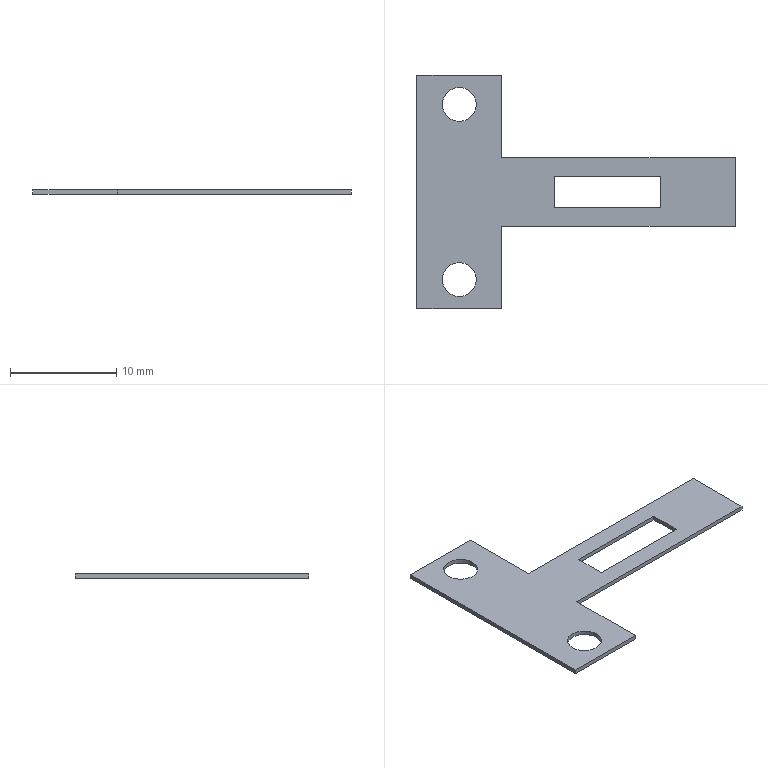Part | SolidWorks | features BaseBody 1 | 1 solid | 18 faces | box 30 x 22 x 0.4115 mm | volume 112.299 mm3 | plane 14 | cylinder 4 | commonest cylinder face diameters 3.2 x4
STEP:
#1=CARTESIAN_POINT('',(5.6,8.25,0.4115));
#2=VERTEX_POINT('',#1);
#3=CARTESIAN_POINT('',(2.4,8.25,0.4115));
#4=VERTEX_POINT('',#3);
#5=CARTESIAN_POINT('',(4.,8.25,0.4115));
#6=DIRECTION('',(0.,0.,-1.));
#7=DIRECTION('',(-1.,0.,0.));
#8=AXIS2_PLACEMENT_3D('',#5,#6,#7);
#9=CIRCLE('',#8,1.6);
#10=EDGE_CURVE('',#2,#4,#9,.T.);
#11=ORIENTED_EDGE('',*,*,#10,.F.);
#12=CARTESIAN_POINT('',(5.6,8.25,0.));
#13=VERTEX_POINT('',#12);
#14=CARTESIAN_POINT('',(5.6,8.25,0.));
#15=DIRECTION('',(0.,0.,-1.));
#16=VECTOR('',#15,1000.);
#17=LINE('',#14,#16);
#18=EDGE_CURVE('',#2,#13,#17,.T.);
#19=ORIENTED_EDGE('',*,*,#18,.T.);
#20=CARTESIAN_POINT('',(2.4,8.25,0.));
#21=VERTEX_POINT('',#20);
#22=CARTESIAN_POINT('',(4.,8.25,0.));
#23=DIRECTION('',(0.,0.,-1.));
#24=DIRECTION('',(-1.,0.,0.));
#25=AXIS2_PLACEMENT_3D('',#22,#23,#24);
#26=CIRCLE('',#25,1.6);
#27=EDGE_CURVE('',#13,#21,#26,.T.);
#28=ORIENTED_EDGE('',*,*,#27,.T.);
#29=CARTESIAN_POINT('',(2.4,8.25,0.));
#30=DIRECTION('',(0.,0.,-1.));
#31=VECTOR('',#30,1000.);
#32=LINE('',#29,#31);
#33=EDGE_CURVE('',#4,#21,#32,.T.);
#34=ORIENTED_EDGE('',*,*,#33,.F.);
#35=EDGE_LOOP('',(#11,#19,#28,#34));
#36=FACE_OUTER_BOUND('',#35,.T.);
#37=CARTESIAN_POINT('',(4.,8.25,0.));
#38=DIRECTION('',(0.,0.,-1.));
#39=DIRECTION('',(-1.,0.,0.));
#40=AXIS2_PLACEMENT_3D('',#37,#38,#39);
#41=CYLINDRICAL_SURFACE('',#40,1.6);
#42=ADVANCED_FACE('',(#36),#41,.F.);
#43=CARTESIAN_POINT('',(5.6,-8.25,0.4115));
#44=VERTEX_POINT('',#43);
#45=CARTESIAN_POINT('',(2.4,-8.25,0.4115));
#46=VERTEX_POINT('',#45);
#47=CARTESIAN_POINT('',(4.,-8.25,0.4115));
#48=DIRECTION('',(0.,0.,-1.));
#49=DIRECTION('',(-1.,0.,0.));
#50=AXIS2_PLACEMENT_3D('',#47,#48,#49);
#51=CIRCLE('',#50,1.6);
#52=EDGE_CURVE('',#44,#46,#51,.T.);
#53=ORIENTED_EDGE('',*,*,#52,.F.);
#54=CARTESIAN_POINT('',(5.6,-8.25,0.));
#55=VERTEX_POINT('',#54);
#56=CARTESIAN_POINT('',(5.6,-8.25,0.));
#57=DIRECTION('',(0.,0.,-1.));
#58=VECTOR('',#57,1000.);
#59=LINE('',#56,#58);
#60=EDGE_CURVE('',#44,#55,#59,.T.);
#61=ORIENTED_EDGE('',*,*,#60,.T.);
#62=CARTESIAN_POINT('',(2.4,-8.25,0.));
#63=VERTEX_POINT('',#62);
#64=CARTESIAN_POINT('',(4.,-8.25,0.));
#65=DIRECTION('',(0.,0.,-1.));
#66=DIRECTION('',(-1.,0.,0.));
#67=AXIS2_PLACEMENT_3D('',#64,#65,#66);
#68=CIRCLE('',#67,1.6);
#69=EDGE_CURVE('',#55,#63,#68,.T.);
#70=ORIENTED_EDGE('',*,*,#69,.T.);
#71=CARTESIAN_POINT('',(2.4,-8.25,0.));
#72=DIRECTION('',(0.,0.,-1.));
#73=VECTOR('',#72,1000.);
#74=LINE('',#71,#73);
#75=EDGE_CURVE('',#46,#63,#74,.T.);
#76=ORIENTED_EDGE('',*,*,#75,.F.);
#77=EDGE_LOOP('',(#53,#61,#70,#76));
#78=FACE_OUTER_BOUND('',#77,.T.);
#79=CARTESIAN_POINT('',(4.,-8.25,0.));
#80=DIRECTION('',(0.,0.,-1.));
#81=DIRECTION('',(-1.,0.,0.));
#82=AXIS2_PLACEMENT_3D('',#79,#80,#81);
#83=CYLINDRICAL_SURFACE('',#82,1.6);
#84=ADVANCED_FACE('',(#78),#83,.F.);
#85=CARTESIAN_POINT('',(4.,8.25,0.));
#86=DIRECTION('',(0.,0.,-1.));
#87=DIRECTION('',(-1.,0.,0.));
#88=AXIS2_PLACEMENT_3D('',#85,#86,#87);
#89=CIRCLE('',#88,1.6);
#90=EDGE_CURVE('',#21,#13,#89,.T.);
#91=ORIENTED_EDGE('',*,*,#90,.F.);
#92=ORIENTED_EDGE('',*,*,#27,.F.);
#93=EDGE_LOOP('',(#91,#92));
#94=FACE_BOUND('',#93,.T.);
#95=CARTESIAN_POINT('',(23.,1.5,0.));
#96=VERTEX_POINT('',#95);
#97=CARTESIAN_POINT('',(23.,-1.5,0.));
#98=VERTEX_POINT('',#97);
#99=CARTESIAN_POINT('',(23.,-11.,0.));
#100=DIRECTION('',(0.,-1.,0.));
#101=VECTOR('',#100,1000.);
#102=LINE('',#99,#101);
#103=EDGE_CURVE('',#96,#98,#102,.T.);
#104=ORIENTED_EDGE('',*,*,#103,.F.);
#105=CARTESIAN_POINT('',(13.,1.5,0.));
#106=VERTEX_POINT('',#105);
#107=CARTESIAN_POINT('',(0.,1.5,0.));
#108=DIRECTION('',(1.,0.,0.));
#109=VECTOR('',#108,1000.);
#110=LINE('',#107,#109);
#111=EDGE_CURVE('',#106,#96,#110,.T.);
#112=ORIENTED_EDGE('',*,*,#111,.F.);
#113=CARTESIAN_POINT('',(13.,-1.5,0.));
#114=VERTEX_POINT('',#113);
#115=CARTESIAN_POINT('',(13.,-11.,0.));
#116=DIRECTION('',(0.,1.,0.));
#117=VECTOR('',#116,1000.);
#118=LINE('',#115,#117);
#119=EDGE_CURVE('',#114,#106,#118,.T.);
#120=ORIENTED_EDGE('',*,*,#119,.F.);
#121=CARTESIAN_POINT('',(0.,-1.5,0.));
#122=DIRECTION('',(-1.,0.,0.));
#123=VECTOR('',#122,1000.);
#124=LINE('',#121,#123);
#125=EDGE_CURVE('',#98,#114,#124,.T.);
#126=ORIENTED_EDGE('',*,*,#125,.F.);
#127=EDGE_LOOP('',(#104,#112,#120,#126));
#128=FACE_BOUND('',#127,.T.);
#129=CARTESIAN_POINT('',(4.,-8.25,0.));
#130=DIRECTION('',(0.,0.,-1.));
#131=DIRECTION('',(-1.,0.,0.));
#132=AXIS2_PLACEMENT_3D('',#129,#130,#131);
#133=CIRCLE('',#132,1.6);
#134=EDGE_CURVE('',#63,#55,#133,.T.);
#135=ORIENTED_EDGE('',*,*,#134,.F.);
#136=ORIENTED_EDGE('',*,*,#69,.F.);
#137=EDGE_LOOP('',(#135,#136));
#138=FACE_BOUND('',#137,.T.);
#139=CARTESIAN_POINT('',(8.,11.,0.));
#140=VERTEX_POINT('',#139);
#141=CARTESIAN_POINT('',(0.,11.,0.));
#142=VERTEX_POINT('',#141);
#143=CARTESIAN_POINT('',(0.,11.,0.));
#144=DIRECTION('',(-1.,0.,0.));
#145=VECTOR('',#144,1000.);
#146=LINE('',#143,#145);
#147=EDGE_CURVE('',#140,#142,#146,.T.);
#148=ORIENTED_EDGE('',*,*,#147,.F.);
#149=CARTESIAN_POINT('',(8.,3.25,0.));
#150=VERTEX_POINT('',#149);
#151=CARTESIAN_POINT('',(8.,-11.,0.));
#152=DIRECTION('',(0.,1.,0.));
#153=VECTOR('',#152,1000.);
#154=LINE('',#151,#153);
#155=EDGE_CURVE('',#150,#140,#154,.T.);
#156=ORIENTED_EDGE('',*,*,#155,.F.);
#157=CARTESIAN_POINT('',(30.,3.25,0.));
#158=VERTEX_POINT('',#157);
#159=CARTESIAN_POINT('',(0.,3.25,0.));
#160=DIRECTION('',(-1.,0.,0.));
#161=VECTOR('',#160,1000.);
#162=LINE('',#159,#161);
#163=EDGE_CURVE('',#158,#150,#162,.T.);
#164=ORIENTED_EDGE('',*,*,#163,.F.);
#165=CARTESIAN_POINT('',(30.,-3.25,0.));
#166=VERTEX_POINT('',#165);
#167=CARTESIAN_POINT('',(30.,-11.,0.));
#168=DIRECTION('',(0.,1.,0.));
#169=VECTOR('',#168,1000.);
#170=LINE('',#167,#169);
#171=EDGE_CURVE('',#166,#158,#170,.T.);
#172=ORIENTED_EDGE('',*,*,#171,.F.);
#173=CARTESIAN_POINT('',(8.,-3.25,0.));
#174=VERTEX_POINT('',#173);
#175=CARTESIAN_POINT('',(0.,-3.25,0.));
#176=DIRECTION('',(1.,0.,0.));
#177=VECTOR('',#176,1000.);
#178=LINE('',#175,#177);
#179=EDGE_CURVE('',#174,#166,#178,.T.);
#180=ORIENTED_EDGE('',*,*,#179,.F.);
#181=CARTESIAN_POINT('',(8.,-11.,0.));
#182=VERTEX_POINT('',#181);
#183=CARTESIAN_POINT('',(8.,-11.,0.));
#184=DIRECTION('',(0.,1.,0.));
#185=VECTOR('',#184,1000.);
#186=LINE('',#183,#185);
#187=EDGE_CURVE('',#182,#174,#186,.T.);
#188=ORIENTED_EDGE('',*,*,#187,.F.);
#189=CARTESIAN_POINT('',(0.,-11.,0.));
#190=VERTEX_POINT('',#189);
#191=CARTESIAN_POINT('',(0.,-11.,0.));
#192=DIRECTION('',(1.,0.,0.));
#193=VECTOR('',#192,1000.);
#194=LINE('',#191,#193);
#195=EDGE_CURVE('',#190,#182,#194,.T.);
#196=ORIENTED_EDGE('',*,*,#195,.F.);
#197=CARTESIAN_POINT('',(0.,-11.,0.));
#198=DIRECTION('',(0.,-1.,0.));
#199=VECTOR('',#198,1000.);
#200=LINE('',#197,#199);
#201=EDGE_CURVE('',#142,#190,#200,.T.);
#202=ORIENTED_EDGE('',*,*,#201,.F.);
#203=EDGE_LOOP('',(#148,#156,#164,#172,#180,#188,#196,#202));
#204=FACE_OUTER_BOUND('',#203,.T.);
#205=CARTESIAN_POINT('',(0.,-11.,0.));
#206=DIRECTION('',(0.,0.,1.));
#207=DIRECTION('',(1.,0.,0.));
#208=AXIS2_PLACEMENT_3D('',#205,#206,#207);
#209=PLANE('',#208);
#210=ADVANCED_FACE('',(#94,#128,#138,#204),#209,.F.);
#211=ORIENTED_EDGE('',*,*,#18,.F.);
#212=CARTESIAN_POINT('',(4.,8.25,0.4115));
#213=DIRECTION('',(0.,0.,-1.));
#214=DIRECTION('',(-1.,0.,0.));
#215=AXIS2_PLACEMENT_3D('',#212,#213,#214);
#216=CIRCLE('',#215,1.6);
#217=EDGE_CURVE('',#4,#2,#216,.T.);
#218=ORIENTED_EDGE('',*,*,#217,.F.);
#219=ORIENTED_EDGE('',*,*,#33,.T.);
#220=ORIENTED_EDGE('',*,*,#90,.T.);
#221=EDGE_LOOP('',(#211,#218,#219,#220));
#222=FACE_OUTER_BOUND('',#221,.T.);
#223=CARTESIAN_POINT('',(4.,8.25,0.));
#224=DIRECTION('',(0.,0.,-1.));
#225=DIRECTION('',(-1.,0.,0.));
#226=AXIS2_PLACEMENT_3D('',#223,#224,#225);
#227=CYLINDRICAL_SURFACE('',#226,1.6);
#228=ADVANCED_FACE('',(#222),#227,.F.);
#229=CARTESIAN_POINT('',(13.,-1.5,0.4115));
#230=VERTEX_POINT('',#229);
#231=CARTESIAN_POINT('',(13.,-1.5,0.));
#232=DIRECTION('',(0.,0.,-1.));
#233=VECTOR('',#232,1000.);
#234=LINE('',#231,#233);
#235=EDGE_CURVE('',#230,#114,#234,.T.);
#236=ORIENTED_EDGE('',*,*,#235,.F.);
#237=CARTESIAN_POINT('',(23.,-1.5,0.4115));
#238=VERTEX_POINT('',#237);
#239=CARTESIAN_POINT('',(23.,-1.5,0.4115));
#240=DIRECTION('',(-1.,0.,0.));
#241=VECTOR('',#240,1000.);
#242=LINE('',#239,#241);
#243=EDGE_CURVE('',#238,#230,#242,.T.);
#244=ORIENTED_EDGE('',*,*,#243,.F.);
#245=CARTESIAN_POINT('',(23.,-1.5,0.));
#246=DIRECTION('',(0.,0.,1.));
#247=VECTOR('',#246,1000.);
#248=LINE('',#245,#247);
#249=EDGE_CURVE('',#98,#238,#248,.T.);
#250=ORIENTED_EDGE('',*,*,#249,.F.);
#251=ORIENTED_EDGE('',*,*,#125,.T.);
#252=EDGE_LOOP('',(#236,#244,#250,#251));
#253=FACE_OUTER_BOUND('',#252,.T.);
#254=CARTESIAN_POINT('',(23.,-1.5,0.));
#255=DIRECTION('',(0.,-1.,0.));
#256=DIRECTION('',(0.,0.,-1.));
#257=AXIS2_PLACEMENT_3D('',#254,#255,#256);
#258=PLANE('',#257);
#259=ADVANCED_FACE('',(#253),#258,.F.);
#260=ORIENTED_EDGE('',*,*,#249,.T.);
#261=CARTESIAN_POINT('',(23.,1.5,0.4115));
#262=VERTEX_POINT('',#261);
#263=CARTESIAN_POINT('',(23.,1.5,0.4115));
#264=DIRECTION('',(0.,-1.,0.));
#265=VECTOR('',#264,1000.);
#266=LINE('',#263,#265);
#267=EDGE_CURVE('',#262,#238,#266,.T.);
#268=ORIENTED_EDGE('',*,*,#267,.F.);
#269=CARTESIAN_POINT('',(23.,1.5,0.));
#270=DIRECTION('',(0.,0.,1.));
#271=VECTOR('',#270,1000.);
#272=LINE('',#269,#271);
#273=EDGE_CURVE('',#96,#262,#272,.T.);
#274=ORIENTED_EDGE('',*,*,#273,.F.);
#275=ORIENTED_EDGE('',*,*,#103,.T.);
#276=EDGE_LOOP('',(#260,#268,#274,#275));
#277=FACE_OUTER_BOUND('',#276,.T.);
#278=CARTESIAN_POINT('',(23.,1.5,0.));
#279=DIRECTION('',(1.,0.,0.));
#280=DIRECTION('',(0.,0.,-1.));
#281=AXIS2_PLACEMENT_3D('',#278,#279,#280);
#282=PLANE('',#281);
#283=ADVANCED_FACE('',(#277),#282,.F.);
#284=ORIENTED_EDGE('',*,*,#273,.T.);
#285=CARTESIAN_POINT('',(13.,1.5,0.4115));
#286=VERTEX_POINT('',#285);
#287=CARTESIAN_POINT('',(13.,1.5,0.4115));
#288=DIRECTION('',(1.,0.,0.));
#289=VECTOR('',#288,1000.);
#290=LINE('',#287,#289);
#291=EDGE_CURVE('',#286,#262,#290,.T.);
#292=ORIENTED_EDGE('',*,*,#291,.F.);
#293=CARTESIAN_POINT('',(13.,1.5,0.));
#294=DIRECTION('',(0.,0.,1.));
#295=VECTOR('',#294,1000.);
#296=LINE('',#293,#295);
#297=EDGE_CURVE('',#106,#286,#296,.T.);
#298=ORIENTED_EDGE('',*,*,#297,.F.);
#299=ORIENTED_EDGE('',*,*,#111,.T.);
#300=EDGE_LOOP('',(#284,#292,#298,#299));
#301=FACE_OUTER_BOUND('',#300,.T.);
#302=CARTESIAN_POINT('',(13.,1.5,0.));
#303=DIRECTION('',(0.,1.,0.));
#304=DIRECTION('',(0.,0.,1.));
#305=AXIS2_PLACEMENT_3D('',#302,#303,#304);
#306=PLANE('',#305);
#307=ADVANCED_FACE('',(#301),#306,.F.);
#308=ORIENTED_EDGE('',*,*,#297,.T.);
#309=CARTESIAN_POINT('',(13.,-1.5,0.4115));
#310=DIRECTION('',(0.,1.,0.));
#311=VECTOR('',#310,1000.);
#312=LINE('',#309,#311);
#313=EDGE_CURVE('',#230,#286,#312,.T.);
#314=ORIENTED_EDGE('',*,*,#313,.F.);
#315=ORIENTED_EDGE('',*,*,#235,.T.);
#316=ORIENTED_EDGE('',*,*,#119,.T.);
#317=EDGE_LOOP('',(#308,#314,#315,#316));
#318=FACE_OUTER_BOUND('',#317,.T.);
#319=CARTESIAN_POINT('',(13.,-1.5,0.));
#320=DIRECTION('',(-1.,0.,0.));
#321=DIRECTION('',(0.,0.,1.));
#322=AXIS2_PLACEMENT_3D('',#319,#320,#321);
#323=PLANE('',#322);
#324=ADVANCED_FACE('',(#318),#323,.F.);
#325=ORIENTED_EDGE('',*,*,#60,.F.);
#326=CARTESIAN_POINT('',(4.,-8.25,0.4115));
#327=DIRECTION('',(0.,0.,-1.));
#328=DIRECTION('',(-1.,0.,0.));
#329=AXIS2_PLACEMENT_3D('',#326,#327,#328);
#330=CIRCLE('',#329,1.6);
#331=EDGE_CURVE('',#46,#44,#330,.T.);
#332=ORIENTED_EDGE('',*,*,#331,.F.);
#333=ORIENTED_EDGE('',*,*,#75,.T.);
#334=ORIENTED_EDGE('',*,*,#134,.T.);
#335=EDGE_LOOP('',(#325,#332,#333,#334));
#336=FACE_OUTER_BOUND('',#335,.T.);
#337=CARTESIAN_POINT('',(4.,-8.25,0.));
#338=DIRECTION('',(0.,0.,-1.));
#339=DIRECTION('',(-1.,0.,0.));
#340=AXIS2_PLACEMENT_3D('',#337,#338,#339);
#341=CYLINDRICAL_SURFACE('',#340,1.6);
#342=ADVANCED_FACE('',(#336),#341,.F.);
#343=CARTESIAN_POINT('',(0.,11.,0.4115));
#344=VERTEX_POINT('',#343);
#345=CARTESIAN_POINT('',(0.,11.,0.));
#346=DIRECTION('',(0.,0.,-1.));
#347=VECTOR('',#346,1000.);
#348=LINE('',#345,#347);
#349=EDGE_CURVE('',#344,#142,#348,.T.);
#350=ORIENTED_EDGE('',*,*,#349,.T.);
#351=ORIENTED_EDGE('',*,*,#201,.T.);
#352=CARTESIAN_POINT('',(0.,-11.,0.4115));
#353=VERTEX_POINT('',#352);
#354=CARTESIAN_POINT('',(0.,-11.,0.));
#355=DIRECTION('',(0.,0.,1.));
#356=VECTOR('',#355,1000.);
#357=LINE('',#354,#356);
#358=EDGE_CURVE('',#190,#353,#357,.T.);
#359=ORIENTED_EDGE('',*,*,#358,.T.);
#360=CARTESIAN_POINT('',(0.,-11.,0.4115));
#361=DIRECTION('',(0.,1.,0.));
#362=VECTOR('',#361,1000.);
#363=LINE('',#360,#362);
#364=EDGE_CURVE('',#353,#344,#363,.T.);
#365=ORIENTED_EDGE('',*,*,#364,.T.);
#366=EDGE_LOOP('',(#350,#351,#359,#365));
#367=FACE_OUTER_BOUND('',#366,.T.);
#368=CARTESIAN_POINT('',(0.,-11.,0.));
#369=DIRECTION('',(-1.,0.,0.));
#370=DIRECTION('',(0.,0.,1.));
#371=AXIS2_PLACEMENT_3D('',#368,#369,#370);
#372=PLANE('',#371);
#373=ADVANCED_FACE('',(#367),#372,.T.);
#374=CARTESIAN_POINT('',(8.,11.,0.4115));
#375=VERTEX_POINT('',#374);
#376=CARTESIAN_POINT('',(8.,11.,0.));
#377=DIRECTION('',(0.,0.,-1.));
#378=VECTOR('',#377,1000.);
#379=LINE('',#376,#378);
#380=EDGE_CURVE('',#375,#140,#379,.T.);
#381=ORIENTED_EDGE('',*,*,#380,.T.);
#382=ORIENTED_EDGE('',*,*,#147,.T.);
#383=ORIENTED_EDGE('',*,*,#349,.F.);
#384=CARTESIAN_POINT('',(0.,11.,0.4115));
#385=DIRECTION('',(1.,0.,0.));
#386=VECTOR('',#385,1000.);
#387=LINE('',#384,#386);
#388=EDGE_CURVE('',#344,#375,#387,.T.);
#389=ORIENTED_EDGE('',*,*,#388,.T.);
#390=EDGE_LOOP('',(#381,#382,#383,#389));
#391=FACE_OUTER_BOUND('',#390,.T.);
#392=CARTESIAN_POINT('',(0.,11.,0.));
#393=DIRECTION('',(0.,1.,0.));
#394=DIRECTION('',(0.,0.,1.));
#395=AXIS2_PLACEMENT_3D('',#392,#393,#394);
#396=PLANE('',#395);
#397=ADVANCED_FACE('',(#391),#396,.T.);
#398=CARTESIAN_POINT('',(8.,3.25,0.4115));
#399=VERTEX_POINT('',#398);
#400=CARTESIAN_POINT('',(8.,3.25,0.));
#401=DIRECTION('',(0.,0.,-1.));
#402=VECTOR('',#401,1000.);
#403=LINE('',#400,#402);
#404=EDGE_CURVE('',#399,#150,#403,.T.);
#405=ORIENTED_EDGE('',*,*,#404,.T.);
#406=ORIENTED_EDGE('',*,*,#155,.T.);
#407=ORIENTED_EDGE('',*,*,#380,.F.);
#408=CARTESIAN_POINT('',(8.,11.,0.4115));
#409=DIRECTION('',(0.,-1.,0.));
#410=VECTOR('',#409,1000.);
#411=LINE('',#408,#410);
#412=EDGE_CURVE('',#375,#399,#411,.T.);
#413=ORIENTED_EDGE('',*,*,#412,.T.);
#414=EDGE_LOOP('',(#405,#406,#407,#413));
#415=FACE_OUTER_BOUND('',#414,.T.);
#416=CARTESIAN_POINT('',(8.,11.,0.));
#417=DIRECTION('',(1.,0.,0.));
#418=DIRECTION('',(0.,0.,-1.));
#419=AXIS2_PLACEMENT_3D('',#416,#417,#418);
#420=PLANE('',#419);
#421=ADVANCED_FACE('',(#415),#420,.T.);
#422=CARTESIAN_POINT('',(30.,3.25,0.4115));
#423=VERTEX_POINT('',#422);
#424=CARTESIAN_POINT('',(30.,3.25,0.));
#425=DIRECTION('',(0.,0.,-1.));
#426=VECTOR('',#425,1000.);
#427=LINE('',#424,#426);
#428=EDGE_CURVE('',#423,#158,#427,.T.);
#429=ORIENTED_EDGE('',*,*,#428,.T.);
#430=ORIENTED_EDGE('',*,*,#163,.T.);
#431=ORIENTED_EDGE('',*,*,#404,.F.);
#432=CARTESIAN_POINT('',(8.,3.25,0.4115));
#433=DIRECTION('',(1.,0.,0.));
#434=VECTOR('',#433,1000.);
#435=LINE('',#432,#434);
#436=EDGE_CURVE('',#399,#423,#435,.T.);
#437=ORIENTED_EDGE('',*,*,#436,.T.);
#438=EDGE_LOOP('',(#429,#430,#431,#437));
#439=FACE_OUTER_BOUND('',#438,.T.);
#440=CARTESIAN_POINT('',(8.,3.25,0.));
#441=DIRECTION('',(0.,1.,0.));
#442=DIRECTION('',(0.,0.,1.));
#443=AXIS2_PLACEMENT_3D('',#440,#441,#442);
#444=PLANE('',#443);
#445=ADVANCED_FACE('',(#439),#444,.T.);
#446=CARTESIAN_POINT('',(30.,-3.25,0.4115));
#447=VERTEX_POINT('',#446);
#448=CARTESIAN_POINT('',(30.,-3.25,0.));
#449=DIRECTION('',(0.,0.,-1.));
#450=VECTOR('',#449,1000.);
#451=LINE('',#448,#450);
#452=EDGE_CURVE('',#447,#166,#451,.T.);
#453=ORIENTED_EDGE('',*,*,#452,.T.);
#454=ORIENTED_EDGE('',*,*,#171,.T.);
#455=ORIENTED_EDGE('',*,*,#428,.F.);
#456=CARTESIAN_POINT('',(30.,3.25,0.4115));
#457=DIRECTION('',(0.,-1.,0.));
#458=VECTOR('',#457,1000.);
#459=LINE('',#456,#458);
#460=EDGE_CURVE('',#423,#447,#459,.T.);
#461=ORIENTED_EDGE('',*,*,#460,.T.);
#462=EDGE_LOOP('',(#453,#454,#455,#461));
#463=FACE_OUTER_BOUND('',#462,.T.);
#464=CARTESIAN_POINT('',(30.,3.25,0.));
#465=DIRECTION('',(1.,0.,0.));
#466=DIRECTION('',(0.,0.,-1.));
#467=AXIS2_PLACEMENT_3D('',#464,#465,#466);
#468=PLANE('',#467);
#469=ADVANCED_FACE('',(#463),#468,.T.);
#470=CARTESIAN_POINT('',(8.,-3.25,0.4115));
#471=VERTEX_POINT('',#470);
#472=CARTESIAN_POINT('',(8.,-3.25,0.));
#473=DIRECTION('',(0.,0.,-1.));
#474=VECTOR('',#473,1000.);
#475=LINE('',#472,#474);
#476=EDGE_CURVE('',#471,#174,#475,.T.);
#477=ORIENTED_EDGE('',*,*,#476,.T.);
#478=ORIENTED_EDGE('',*,*,#179,.T.);
#479=ORIENTED_EDGE('',*,*,#452,.F.);
#480=CARTESIAN_POINT('',(30.,-3.25,0.4115));
#481=DIRECTION('',(-1.,0.,0.));
#482=VECTOR('',#481,1000.);
#483=LINE('',#480,#482);
#484=EDGE_CURVE('',#447,#471,#483,.T.);
#485=ORIENTED_EDGE('',*,*,#484,.T.);
#486=EDGE_LOOP('',(#477,#478,#479,#485));
#487=FACE_OUTER_BOUND('',#486,.T.);
#488=CARTESIAN_POINT('',(30.,-3.25,0.));
#489=DIRECTION('',(0.,-1.,0.));
#490=DIRECTION('',(0.,0.,-1.));
#491=AXIS2_PLACEMENT_3D('',#488,#489,#490);
#492=PLANE('',#491);
#493=ADVANCED_FACE('',(#487),#492,.T.);
#494=CARTESIAN_POINT('',(8.,-11.,0.4115));
#495=VERTEX_POINT('',#494);
#496=CARTESIAN_POINT('',(8.,-11.,0.));
#497=DIRECTION('',(0.,0.,-1.));
#498=VECTOR('',#497,1000.);
#499=LINE('',#496,#498);
#500=EDGE_CURVE('',#495,#182,#499,.T.);
#501=ORIENTED_EDGE('',*,*,#500,.T.);
#502=ORIENTED_EDGE('',*,*,#187,.T.);
#503=ORIENTED_EDGE('',*,*,#476,.F.);
#504=CARTESIAN_POINT('',(8.,-3.25,0.4115));
#505=DIRECTION('',(0.,-1.,0.));
#506=VECTOR('',#505,1000.);
#507=LINE('',#504,#506);
#508=EDGE_CURVE('',#471,#495,#507,.T.);
#509=ORIENTED_EDGE('',*,*,#508,.T.);
#510=EDGE_LOOP('',(#501,#502,#503,#509));
#511=FACE_OUTER_BOUND('',#510,.T.);
#512=CARTESIAN_POINT('',(8.,-3.25,0.));
#513=DIRECTION('',(1.,0.,0.));
#514=DIRECTION('',(0.,0.,-1.));
#515=AXIS2_PLACEMENT_3D('',#512,#513,#514);
#516=PLANE('',#515);
#517=ADVANCED_FACE('',(#511),#516,.T.);
#518=ORIENTED_EDGE('',*,*,#358,.F.);
#519=ORIENTED_EDGE('',*,*,#195,.T.);
#520=ORIENTED_EDGE('',*,*,#500,.F.);
#521=CARTESIAN_POINT('',(8.,-11.,0.4115));
#522=DIRECTION('',(-1.,0.,0.));
#523=VECTOR('',#522,1000.);
#524=LINE('',#521,#523);
#525=EDGE_CURVE('',#495,#353,#524,.T.);
#526=ORIENTED_EDGE('',*,*,#525,.T.);
#527=EDGE_LOOP('',(#518,#519,#520,#526));
#528=FACE_OUTER_BOUND('',#527,.T.);
#529=CARTESIAN_POINT('',(8.,-11.,0.));
#530=DIRECTION('',(0.,-1.,0.));
#531=DIRECTION('',(0.,0.,-1.));
#532=AXIS2_PLACEMENT_3D('',#529,#530,#531);
#533=PLANE('',#532);
#534=ADVANCED_FACE('',(#528),#533,.T.);
#535=ORIENTED_EDGE('',*,*,#217,.T.);
#536=ORIENTED_EDGE('',*,*,#10,.T.);
#537=EDGE_LOOP('',(#535,#536));
#538=FACE_BOUND('',#537,.T.);
#539=ORIENTED_EDGE('',*,*,#267,.T.);
#540=ORIENTED_EDGE('',*,*,#243,.T.);
#541=ORIENTED_EDGE('',*,*,#313,.T.);
#542=ORIENTED_EDGE('',*,*,#291,.T.);
#543=EDGE_LOOP('',(#539,#540,#541,#542));
#544=FACE_BOUND('',#543,.T.);
#545=ORIENTED_EDGE('',*,*,#331,.T.);
#546=ORIENTED_EDGE('',*,*,#52,.T.);
#547=EDGE_LOOP('',(#545,#546));
#548=FACE_BOUND('',#547,.T.);
#549=ORIENTED_EDGE('',*,*,#388,.F.);
#550=ORIENTED_EDGE('',*,*,#364,.F.);
#551=ORIENTED_EDGE('',*,*,#525,.F.);
#552=ORIENTED_EDGE('',*,*,#508,.F.);
#553=ORIENTED_EDGE('',*,*,#484,.F.);
#554=ORIENTED_EDGE('',*,*,#460,.F.);
#555=ORIENTED_EDGE('',*,*,#436,.F.);
#556=ORIENTED_EDGE('',*,*,#412,.F.);
#557=EDGE_LOOP('',(#549,#550,#551,#552,#553,#554,#555,#556));
#558=FACE_OUTER_BOUND('',#557,.T.);
#559=CARTESIAN_POINT('',(0.,-11.,0.4115));
#560=DIRECTION('',(0.,0.,1.));
#561=DIRECTION('',(1.,0.,0.));
#562=AXIS2_PLACEMENT_3D('',#559,#560,#561);
#563=PLANE('',#562);
#564=ADVANCED_FACE('',(#538,#544,#548,#558),#563,.T.);
#565=CLOSED_SHELL('',(#42,#84,#210,#228,#259,#283,#307,#324,#342,#373,#397,#421,#445,#469,#493,#517,#534,#564));
#566=MANIFOLD_SOLID_BREP('',#565);
#567=CARTESIAN_POINT('',(0.,0.,0.));
#568=DIRECTION('',(0.,0.,1.));
#569=DIRECTION('',(1.,0.,0.));
#570=AXIS2_PLACEMENT_3D('',#567,#568,#569);
#571=(LENGTH_UNIT()NAMED_UNIT(*)SI_UNIT(.MILLI.,.METRE.));
#572=UNCERTAINTY_MEASURE_WITH_UNIT(LENGTH_MEASURE(0.00001),#571,'','');
#573=(NAMED_UNIT(*)PLANE_ANGLE_UNIT()SI_UNIT($,.RADIAN.));
#574=(NAMED_UNIT(*)SI_UNIT($,.STERADIAN.)SOLID_ANGLE_UNIT());
#575=(GEOMETRIC_REPRESENTATION_CONTEXT(3)GLOBAL_UNCERTAINTY_ASSIGNED_CONTEXT((#572))GLOBAL_UNIT_ASSIGNED_CONTEXT((#571,#573,#574))REPRESENTATION_CONTEXT('',''));
#576=ADVANCED_BREP_SHAPE_REPRESENTATION('',(#566,#570),#575);